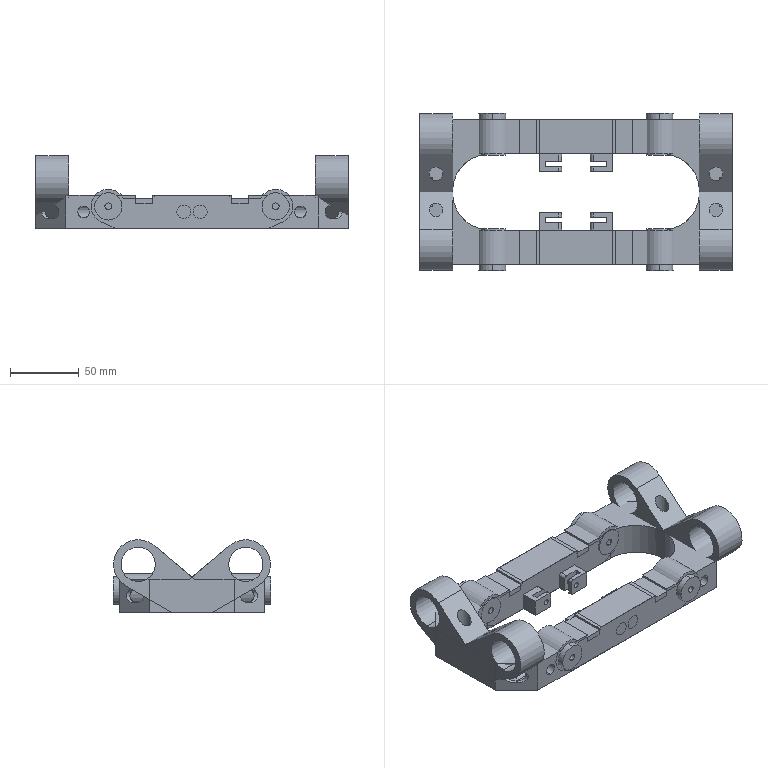NC program | Mastercam | posted with a generic post | part box 228 x 114.503 x 53 mm
Lines 3036 to 3656 of 11407:
(6 CHM |TOOL - 7|DIA. OFF. - 7|LEN. - 7|TOOL DIA. - 6.)
N6154 T7 M6
N6156 G0 G54 G90 X129.548 Y-5.75 C0. B0. S6000 M3
N6158 G43 H7 Z62.5
N6160 G81 G98 Z36.8 R39.5 F300.
N6162 G80
N6164 M5
N6166 G0 G28 G91 Z0.
N6168 G28
N6170 M01
N6172 G0 G17 G40 G80 G90 G94 G98
N6174 G0 G28 G91 Z0.
(12 FEM |TOOL - 12|DIA. OFF. - 12|LEN. - 12|TOOL DIA. - 12.)
N6176 T12 M6
N6178 G0 G54 G90 X164.238 Y26.324 C0. B0. S6000 M3
N6180 G43 H12 Z76.
N6182 Z31.
N6184 G1 Z25.5 F600.
N6186 X165.204 Y23.483 F6000.
N6188 G3 X168.044 Y21.449 I2.84 J.966
N6190 X169.01 Y21.609 J3.
N6192 G2 X175. Y22.6 I5.99 J-17.609
N6194 X193.6 Y4. J-18.6
N6196 X182.692 Y-12.935 I-18.6
N6198 G1 X172.523 Y-17.554
N6200 G3 X170.764 Y-20.285 I1.24 J-2.731
N6202 X171.032 Y-21.526 I2.999
N6204 G1 X172.272 Y-24.257
N6206 Z25. F600.
N6208 X171.032 Y-21.526 F6000.
N6210 G2 X170.763 Y-20.285 I2.731 J1.241
N6212 X172.523 Y-17.554 I3.
N6214 G1 X182.692 Y-12.935
N6216 G3 X193.6 Y4. I-7.692 J16.935
N6218 X175. Y22.6 I-18.6
N6220 X169.01 Y21.609 J-18.6
N6222 G2 X168.044 Y21.449 I-.966 J2.84
N6224 X165.204 Y23.483 J3.
N6226 G1 X164.238 Y26.324
N6228 Z24.5 F600.
N6230 X165.204 Y23.483 F6000.
N6232 G3 X168.044 Y21.449 I2.84 J.966
N6234 X169.01 Y21.609 J3.
N6236 G2 X175. Y22.6 I5.99 J-17.609
N6238 X193.6 Y4. J-18.6
N6240 X182.692 Y-12.935 I-18.6
N6242 G1 X172.523 Y-17.554
N6244 G3 X170.764 Y-20.285 I1.24 J-2.731
N6246 X171.032 Y-21.526 I2.999
N6248 G1 X172.272 Y-24.257
N6250 Z24. F600.
N6252 X171.032 Y-21.526 F6000.
N6254 G2 X170.763 Y-20.285 I2.731 J1.241
N6256 X172.523 Y-17.554 I3.
N6258 G1 X182.692 Y-12.935
N6260 G3 X193.6 Y4. I-7.692 J16.935
N6262 X175. Y22.6 I-18.6
N6264 X169.01 Y21.609 J-18.6
N6266 G2 X168.044 Y21.449 I-.966 J2.84
N6268 X165.204 Y23.483 J3.
N6270 G1 X164.238 Y26.324
N6272 Z23.5 F600.
N6274 X165.204 Y23.483 F6000.
N6276 G3 X168.044 Y21.449 I2.84 J.966
N6278 X169.01 Y21.609 J3.
N6280 G2 X175. Y22.6 I5.99 J-17.609
N6282 X193.6 Y4. J-18.6
N6284 X182.692 Y-12.935 I-18.6
N6286 G1 X172.523 Y-17.554
N6288 G3 X170.764 Y-20.285 I1.24 J-2.731
N6290 X171.032 Y-21.526 I2.999
N6292 G1 X172.272 Y-24.257
N6294 Z23. F600.
N6296 X171.032 Y-21.526 F6000.
N6298 G2 X170.763 Y-20.285 I2.731 J1.241
N6300 X172.523 Y-17.554 I3.
N6302 G1 X182.692 Y-12.935
N6304 G3 X193.6 Y4. I-7.692 J16.935
N6306 X175. Y22.6 I-18.6
N6308 X169.01 Y21.609 J-18.6
N6310 G2 X168.044 Y21.449 I-.966 J2.84
N6312 X165.204 Y23.483 J3.
N6314 G1 X164.238 Y26.324
N6316 Z22.5 F600.
N6318 X165.204 Y23.483 F6000.
N6320 G3 X168.044 Y21.449 I2.84 J.966
N6322 X169.01 Y21.609 J3.
N6324 G2 X175. Y22.6 I5.99 J-17.609
N6326 X193.6 Y4. J-18.6
N6328 X182.692 Y-12.935 I-18.6
N6330 G1 X172.523 Y-17.554
N6332 G3 X170.764 Y-20.285 I1.24 J-2.731
N6334 X171.032 Y-21.526 I2.999
N6336 G1 X172.272 Y-24.257
N6338 Z22. F600.
N6340 X171.032 Y-21.526 F6000.
N6342 G2 X170.763 Y-20.285 I2.731 J1.241
N6344 X172.523 Y-17.554 I3.
N6346 G1 X182.692 Y-12.935
N6348 G3 X193.6 Y4. I-7.692 J16.935
N6350 X175. Y22.6 I-18.6
N6352 X169.01 Y21.609 J-18.6
N6354 G2 X168.044 Y21.449 I-.966 J2.84
N6356 X165.204 Y23.483 J3.
N6358 G1 X164.238 Y26.324
N6360 Z21.5 F600.
N6362 X165.204 Y23.483 F6000.
N6364 G3 X168.044 Y21.449 I2.84 J.966
N6366 X169.01 Y21.609 J3.
N6368 G2 X175. Y22.6 I5.99 J-17.609
N6370 X193.6 Y4. J-18.6
N6372 X182.692 Y-12.935 I-18.6
N6374 G1 X172.523 Y-17.554
N6376 G3 X170.764 Y-20.285 I1.24 J-2.731
N6378 X171.032 Y-21.526 I2.999
N6380 G1 X172.272 Y-24.257
N6382 Z21. F600.
N6384 X171.032 Y-21.526 F6000.
N6386 G2 X170.763 Y-20.285 I2.731 J1.241
N6388 X172.523 Y-17.554 I3.
N6390 G1 X182.692 Y-12.935
N6392 G3 X193.6 Y4. I-7.692 J16.935
N6394 X175. Y22.6 I-18.6
N6396 X169.01 Y21.609 J-18.6
N6398 G2 X168.044 Y21.449 I-.966 J2.84
N6400 X165.204 Y23.483 J3.
N6402 G1 X164.238 Y26.324
N6404 Z20.5 F600.
N6406 X165.204 Y23.483 F6000.
N6408 G3 X168.044 Y21.449 I2.84 J.966
N6410 X169.01 Y21.609 J3.
N6412 G2 X175. Y22.6 I5.99 J-17.609
N6414 X193.6 Y4. J-18.6
N6416 X182.692 Y-12.935 I-18.6
N6418 G1 X172.523 Y-17.554
N6420 G3 X170.764 Y-20.285 I1.24 J-2.731
N6422 X171.032 Y-21.526 I2.999
N6424 G1 X172.272 Y-24.257
N6426 Z20. F600.
N6428 X171.032 Y-21.526 F6000.
N6430 G2 X170.763 Y-20.285 I2.731 J1.241
N6432 X172.523 Y-17.554 I3.
N6434 G1 X182.692 Y-12.935
N6436 G3 X193.6 Y4. I-7.692 J16.935
N6438 X175. Y22.6 I-18.6
N6440 X169.01 Y21.609 J-18.6
N6442 G2 X168.044 Y21.449 I-.966 J2.84
N6444 X165.204 Y23.483 J3.
N6446 G1 X164.238 Y26.324
N6448 Z19.5 F600.
N6450 X165.204 Y23.483 F6000.
N6452 G3 X168.044 Y21.449 I2.84 J.966
N6454 X169.01 Y21.609 J3.
N6456 G2 X175. Y22.6 I5.99 J-17.609
N6458 X193.6 Y4. J-18.6
N6460 X182.692 Y-12.935 I-18.6
N6462 G1 X172.523 Y-17.554
N6464 G3 X170.764 Y-20.285 I1.24 J-2.731
N6466 X171.032 Y-21.526 I2.999
N6468 G1 X172.272 Y-24.257
N6470 Z19. F600.
N6472 X171.032 Y-21.526 F6000.
N6474 G2 X170.763 Y-20.285 I2.731 J1.241
N6476 X172.523 Y-17.554 I3.
N6478 G1 X182.692 Y-12.935
N6480 G3 X193.6 Y4. I-7.692 J16.935
N6482 X175. Y22.6 I-18.6
N6484 X169.01 Y21.609 J-18.6
N6486 G2 X168.044 Y21.449 I-.966 J2.84
N6488 X165.204 Y23.483 J3.
N6490 G1 X164.238 Y26.324
N6492 Z18.5 F600.
N6494 X165.204 Y23.483 F6000.
N6496 G3 X168.044 Y21.449 I2.84 J.966
N6498 X169.01 Y21.609 J3.
N6500 G2 X175. Y22.6 I5.99 J-17.609
N6502 X193.6 Y4. J-18.6
N6504 X182.692 Y-12.935 I-18.6
N6506 G1 X172.523 Y-17.554
N6508 G3 X170.764 Y-20.285 I1.24 J-2.731
N6510 X171.032 Y-21.526 I2.999
N6512 G1 X172.272 Y-24.257
N6514 Z18. F600.
N6516 X171.032 Y-21.526 F6000.
N6518 G2 X170.763 Y-20.285 I2.731 J1.241
N6520 X172.523 Y-17.554 I3.
N6522 G1 X182.692 Y-12.935
N6524 G3 X193.6 Y4. I-7.692 J16.935
N6526 X175. Y22.6 I-18.6
N6528 X169.01 Y21.609 J-18.6
N6530 G2 X168.044 Y21.449 I-.966 J2.84
N6532 X165.204 Y23.483 J3.
N6534 G1 X164.238 Y26.324
N6536 Z17.5 F600.
N6538 X165.204 Y23.483 F6000.
N6540 G3 X168.044 Y21.449 I2.84 J.966
N6542 X169.01 Y21.609 J3.
N6544 G2 X175. Y22.6 I5.99 J-17.609
N6546 X193.6 Y4. J-18.6
N6548 X182.692 Y-12.935 I-18.6
N6550 G1 X172.523 Y-17.554
N6552 G3 X170.764 Y-20.285 I1.24 J-2.731
N6554 X171.032 Y-21.526 I2.999
N6556 G1 X172.272 Y-24.257
N6558 Z17. F600.
N6560 X171.032 Y-21.526 F6000.
N6562 G2 X170.763 Y-20.285 I2.731 J1.241
N6564 X172.523 Y-17.554 I3.
N6566 G1 X182.692 Y-12.935
N6568 G3 X193.6 Y4. I-7.692 J16.935
N6570 X175. Y22.6 I-18.6
N6572 X169.01 Y21.609 J-18.6
N6574 G2 X168.044 Y21.449 I-.966 J2.84
N6576 X165.204 Y23.483 J3.
N6578 G1 X164.238 Y26.324
N6580 Z16.5 F600.
N6582 X165.204 Y23.483 F6000.
N6584 G3 X168.044 Y21.449 I2.84 J.966
N6586 X169.01 Y21.609 J3.
N6588 G2 X175. Y22.6 I5.99 J-17.609
N6590 X193.6 Y4. J-18.6
N6592 X182.692 Y-12.935 I-18.6
N6594 G1 X172.523 Y-17.554
N6596 G3 X170.764 Y-20.285 I1.24 J-2.731
N6598 X171.032 Y-21.526 I2.999
N6600 G1 X172.272 Y-24.257
N6602 Z16. F600.
N6604 X171.032 Y-21.526 F6000.
N6606 G2 X170.763 Y-20.285 I2.731 J1.241
N6608 X172.523 Y-17.554 I3.
N6610 G1 X182.692 Y-12.935
N6612 G3 X193.6 Y4. I-7.692 J16.935
N6614 X175. Y22.6 I-18.6
N6616 X169.01 Y21.609 J-18.6
N6618 G2 X168.044 Y21.449 I-.966 J2.84
N6620 X165.204 Y23.483 J3.
N6622 G1 X164.238 Y26.324
N6624 Z15.5 F600.
N6626 X165.204 Y23.483 F6000.
N6628 G3 X168.044 Y21.449 I2.84 J.966
N6630 X169.01 Y21.609 J3.
N6632 G2 X175. Y22.6 I5.99 J-17.609
N6634 X193.6 Y4. J-18.6
N6636 X182.692 Y-12.935 I-18.6
N6638 G1 X172.523 Y-17.554
N6640 G3 X170.764 Y-20.285 I1.24 J-2.731
N6642 X171.032 Y-21.526 I2.999
N6644 G1 X172.272 Y-24.257
N6646 Z15. F600.
N6648 X171.032 Y-21.526 F6000.
N6650 G2 X170.763 Y-20.285 I2.731 J1.241
N6652 X172.523 Y-17.554 I3.
N6654 G1 X182.692 Y-12.935
N6656 G3 X193.6 Y4. I-7.692 J16.935
N6658 X175. Y22.6 I-18.6
N6660 X169.01 Y21.609 J-18.6
N6662 G2 X168.044 Y21.449 I-.966 J2.84
N6664 X165.204 Y23.483 J3.
N6666 G1 X164.238 Y26.324
N6668 Z14.5 F600.
N6670 X165.204 Y23.483 F6000.
N6672 G3 X168.044 Y21.449 I2.84 J.966
N6674 X169.01 Y21.609 J3.
N6676 G2 X175. Y22.6 I5.99 J-17.609
N6678 X193.6 Y4. J-18.6
N6680 X182.692 Y-12.935 I-18.6
N6682 G1 X172.523 Y-17.554
N6684 G3 X170.764 Y-20.285 I1.24 J-2.731
N6686 X171.032 Y-21.526 I2.999
N6688 G1 X172.272 Y-24.257
N6690 Z14. F600.
N6692 X171.032 Y-21.526 F6000.
N6694 G2 X170.763 Y-20.285 I2.731 J1.241
N6696 X172.523 Y-17.554 I3.
N6698 G1 X182.692 Y-12.935
N6700 G3 X193.6 Y4. I-7.692 J16.935
N6702 X175. Y22.6 I-18.6
N6704 X169.01 Y21.609 J-18.6
N6706 G2 X168.044 Y21.449 I-.966 J2.84
N6708 X165.204 Y23.483 J3.
N6710 G1 X164.238 Y26.324
N6712 Z13.5 F600.
N6714 X165.204 Y23.483 F6000.
N6716 G3 X168.044 Y21.449 I2.84 J.966
N6718 X169.01 Y21.609 J3.
N6720 G2 X175. Y22.6 I5.99 J-17.609
N6722 X193.6 Y4. J-18.6
N6724 X182.692 Y-12.935 I-18.6
N6726 G1 X172.523 Y-17.554
N6728 G3 X170.764 Y-20.285 I1.24 J-2.731
N6730 X171.032 Y-21.526 I2.999
N6732 G1 X172.272 Y-24.257
N6734 Z13. F600.
N6736 X171.032 Y-21.526 F6000.
N6738 G2 X170.763 Y-20.285 I2.731 J1.241
N6740 X172.523 Y-17.554 I3.
N6742 G1 X182.692 Y-12.935
N6744 G3 X193.6 Y4. I-7.692 J16.935
N6746 X175. Y22.6 I-18.6
N6748 X169.01 Y21.609 J-18.6
N6750 G2 X168.044 Y21.449 I-.966 J2.84
N6752 X165.204 Y23.483 J3.
N6754 G1 X164.238 Y26.324
N6756 Z12.5 F600.
N6758 X165.204 Y23.483 F6000.
N6760 G3 X168.044 Y21.449 I2.84 J.966
N6762 X169.01 Y21.609 J3.
N6764 G2 X175. Y22.6 I5.99 J-17.609
N6766 X193.6 Y4. J-18.6
N6768 X182.692 Y-12.935 I-18.6
N6770 G1 X172.523 Y-17.554
N6772 G3 X170.764 Y-20.285 I1.24 J-2.731
N6774 X171.032 Y-21.526 I2.999
N6776 G1 X172.272 Y-24.257
N6778 Z12. F600.
N6780 X171.032 Y-21.526 F6000.
N6782 G2 X170.763 Y-20.285 I2.731 J1.241
N6784 X172.523 Y-17.554 I3.
N6786 G1 X182.692 Y-12.935
N6788 G3 X193.6 Y4. I-7.692 J16.935
N6790 X175. Y22.6 I-18.6
N6792 X169.01 Y21.609 J-18.6
N6794 G2 X168.044 Y21.449 I-.966 J2.84
N6796 X165.204 Y23.483 J3.
N6798 G1 X164.238 Y26.324
N6800 Z11.5 F600.
N6802 X165.204 Y23.483 F6000.
N6804 G3 X168.044 Y21.449 I2.84 J.966
N6806 X169.01 Y21.609 J3.
N6808 G2 X175. Y22.6 I5.99 J-17.609
N6810 X193.6 Y4. J-18.6
N6812 X182.692 Y-12.935 I-18.6
N6814 G1 X172.523 Y-17.554
N6816 G3 X170.764 Y-20.285 I1.24 J-2.731
N6818 X171.032 Y-21.526 I2.999
N6820 G1 X172.272 Y-24.257
N6822 Z11. F600.
N6824 X171.032 Y-21.526 F6000.
N6826 G2 X170.763 Y-20.285 I2.731 J1.241
N6828 X172.523 Y-17.554 I3.
N6830 G1 X182.692 Y-12.935
N6832 G3 X193.6 Y4. I-7.692 J16.935
N6834 X175. Y22.6 I-18.6
N6836 X169.01 Y21.609 J-18.6
N6838 G2 X168.044 Y21.449 I-.966 J2.84
N6840 X165.204 Y23.483 J3.
N6842 G1 X164.238 Y26.324
N6844 Z10.5 F600.
N6846 X165.204 Y23.483 F6000.
N6848 G3 X168.044 Y21.449 I2.84 J.966
N6850 X169.01 Y21.609 J3.
N6852 G2 X175. Y22.6 I5.99 J-17.609
N6854 X193.6 Y4. J-18.6
N6856 X182.692 Y-12.935 I-18.6
N6858 G1 X172.523 Y-17.554
N6860 G3 X170.764 Y-20.285 I1.24 J-2.731
N6862 X171.032 Y-21.526 I2.999
N6864 G1 X172.272 Y-24.257
N6866 Z10. F600.
N6868 X171.032 Y-21.526 F6000.
N6870 G2 X170.763 Y-20.285 I2.731 J1.241
N6872 X172.523 Y-17.554 I3.
N6874 G1 X182.692 Y-12.935
N6876 G3 X193.6 Y4. I-7.692 J16.935
N6878 X175. Y22.6 I-18.6
N6880 X169.01 Y21.609 J-18.6
N6882 G2 X168.044 Y21.449 I-.966 J2.84
N6884 X165.204 Y23.483 J3.
N6886 G1 X164.238 Y26.324
N6888 Z9.5 F600.
N6890 X165.204 Y23.483 F6000.
N6892 G3 X168.044 Y21.449 I2.84 J.966
N6894 X169.01 Y21.609 J3.
N6896 G2 X175. Y22.6 I5.99 J-17.609
N6898 X193.6 Y4. J-18.6
N6900 X182.692 Y-12.935 I-18.6
N6902 G1 X172.523 Y-17.554
N6904 G3 X170.764 Y-20.285 I1.24 J-2.731
N6906 X171.032 Y-21.526 I2.999
N6908 G1 X172.272 Y-24.257
N6910 Z9. F600.
N6912 X171.032 Y-21.526 F6000.
N6914 G2 X170.763 Y-20.285 I2.731 J1.241
N6916 X172.523 Y-17.554 I3.
N6918 G1 X182.692 Y-12.935
N6920 G3 X193.6 Y4. I-7.692 J16.935
N6922 X175. Y22.6 I-18.6
N6924 X169.01 Y21.609 J-18.6
N6926 G2 X168.044 Y21.449 I-.966 J2.84
N6928 X165.204 Y23.483 J3.
N6930 G1 X164.238 Y26.324
N6932 Z8.5 F600.
N6934 X165.204 Y23.483 F6000.
N6936 G3 X168.044 Y21.449 I2.84 J.966
N6938 X169.01 Y21.609 J3.
N6940 G2 X175. Y22.6 I5.99 J-17.609
N6942 X193.6 Y4. J-18.6
N6944 X182.692 Y-12.935 I-18.6
N6946 G1 X172.523 Y-17.554
N6948 G3 X170.764 Y-20.285 I1.24 J-2.731
N6950 X171.032 Y-21.526 I2.999
N6952 G1 X172.272 Y-24.257
N6954 Z8. F600.
N6956 X171.032 Y-21.526 F6000.
N6958 G2 X170.763 Y-20.285 I2.731 J1.241
N6960 X172.523 Y-17.554 I3.
N6962 G1 X182.692 Y-12.935
N6964 G3 X193.6 Y4. I-7.692 J16.935
N6966 X175. Y22.6 I-18.6
N6968 X169.01 Y21.609 J-18.6
N6970 G2 X168.044 Y21.449 I-.966 J2.84
N6972 X165.204 Y23.483 J3.
N6974 G1 X164.238 Y26.324
N6976 Z7.5 F600.
N6978 X165.204 Y23.483 F6000.
N6980 G3 X168.044 Y21.449 I2.84 J.966
N6982 X169.01 Y21.609 J3.
N6984 G2 X175. Y22.6 I5.99 J-17.609
N6986 X193.6 Y4. J-18.6
N6988 X182.692 Y-12.935 I-18.6
N6990 G1 X172.523 Y-17.554
N6992 G3 X170.764 Y-20.285 I1.24 J-2.731
N6994 X171.032 Y-21.526 I2.999
N6996 G1 X172.272 Y-24.257
N6998 Z7. F600.
N7000 X171.032 Y-21.526 F6000.
N7002 G2 X170.763 Y-20.285 I2.731 J1.241
N7004 X172.523 Y-17.554 I3.
N7006 G1 X182.692 Y-12.935
N7008 G3 X193.6 Y4. I-7.692 J16.935
N7010 X175. Y22.6 I-18.6
N7012 X169.01 Y21.609 J-18.6
N7014 G2 X168.044 Y21.449 I-.966 J2.84
N7016 X165.204 Y23.483 J3.
N7018 G1 X164.238 Y26.324
N7020 Z6.5 F600.
N7022 X165.204 Y23.483 F6000.
N7024 G3 X168.044 Y21.449 I2.84 J.966
N7026 X169.01 Y21.609 J3.
N7028 G2 X175. Y22.6 I5.99 J-17.609
N7030 X193.6 Y4. J-18.6
N7032 X182.692 Y-12.935 I-18.6
N7034 G1 X172.523 Y-17.554
N7036 G3 X170.764 Y-20.285 I1.24 J-2.731
N7038 X171.032 Y-21.526 I2.999
N7040 G1 X172.272 Y-24.257
N7042 Z6. F600.
N7044 X171.032 Y-21.526 F6000.
N7046 G2 X170.763 Y-20.285 I2.731 J1.241
N7048 X172.523 Y-17.554 I3.
N7050 G1 X182.692 Y-12.935
N7052 G3 X193.6 Y4. I-7.692 J16.935
N7054 X175. Y22.6 I-18.6
N7056 X169.01 Y21.609 J-18.6
N7058 G2 X168.044 Y21.449 I-.966 J2.84
N7060 X165.204 Y23.483 J3.
N7062 G1 X164.238 Y26.324
N7064 Z5.5 F600.
N7066 X165.204 Y23.483 F6000.
N7068 G3 X168.044 Y21.449 I2.84 J.966
N7070 X169.01 Y21.609 J3.
N7072 G2 X175. Y22.6 I5.99 J-17.609
N7074 X193.6 Y4. J-18.6
N7076 X182.692 Y-12.935 I-18.6
N7078 G1 X172.523 Y-17.554
N7080 G3 X170.764 Y-20.285 I1.24 J-2.731
N7082 X171.032 Y-21.526 I2.999
N7084 G1 X172.272 Y-24.257
N7086 Z5. F600.
N7088 X171.032 Y-21.526 F6000.
N7090 G2 X170.763 Y-20.285 I2.731 J1.241
N7092 X172.523 Y-17.554 I3.
N7094 G1 X182.692 Y-12.935
N7096 G3 X193.6 Y4. I-7.692 J16.935
N7098 X175. Y22.6 I-18.6
N7100 X169.01 Y21.609 J-18.6
N7102 G2 X168.044 Y21.449 I-.966 J2.84
N7104 X165.204 Y23.483 J3.
N7106 G1 X164.238 Y26.324
N7108 Z4.5 F600.
N7110 X165.204 Y23.483 F6000.
N7112 G3 X168.044 Y21.449 I2.84 J.966
N7114 X169.01 Y21.609 J3.
N7116 G2 X175. Y22.6 I5.99 J-17.609
N7118 X193.6 Y4. J-18.6
N7120 X182.692 Y-12.935 I-18.6
N7122 G1 X172.523 Y-17.554
N7124 G3 X170.764 Y-20.285 I1.24 J-2.731
N7126 X171.032 Y-21.526 I2.999
N7128 G1 X172.272 Y-24.257
N7130 Z4. F600.
N7132 X171.032 Y-21.526 F6000.
N7134 G2 X170.763 Y-20.285 I2.731 J1.241
N7136 X172.523 Y-17.554 I3.
N7138 G1 X182.692 Y-12.935
N7140 G3 X193.6 Y4. I-7.692 J16.935
N7142 X175. Y22.6 I-18.6
N7144 X169.01 Y21.609 J-18.6
N7146 G2 X168.044 Y21.449 I-.966 J2.84
N7148 X165.204 Y23.483 J3.
N7150 G1 X164.238 Y26.324
N7152 Z3.5 F600.
N7154 X165.204 Y23.483 F6000.
N7156 G3 X168.044 Y21.449 I2.84 J.966
N7158 X169.01 Y21.609 J3.
N7160 G2 X175. Y22.6 I5.99 J-17.609
N7162 X193.6 Y4. J-18.6
N7164 X182.692 Y-12.935 I-18.6
N7166 G1 X172.523 Y-17.554
N7168 G3 X170.764 Y-20.285 I1.24 J-2.731
N7170 X171.032 Y-21.526 I2.999
N7172 G1 X172.272 Y-24.257
N7174 Z3. F600.
N7176 X171.032 Y-21.526 F6000.
N7178 G2 X170.763 Y-20.285 I2.731 J1.241
N7180 X172.523 Y-17.554 I3.
N7182 G1 X182.692 Y-12.935
N7184 G3 X193.6 Y4. I-7.692 J16.935
N7186 X175. Y22.6 I-18.6
N7188 X169.01 Y21.609 J-18.6
N7190 G2 X168.044 Y21.449 I-.966 J2.84
N7192 X165.204 Y23.483 J3.
N7194 G1 X164.238 Y26.324
N7196 Z2.5 F600.
N7198 X165.204 Y23.483 F6000.
N7200 G3 X168.044 Y21.449 I2.84 J.966
N7202 X169.01 Y21.609 J3.
N7204 G2 X175. Y22.6 I5.99 J-17.609
N7206 X193.6 Y4. J-18.6
N7208 X182.692 Y-12.935 I-18.6
N7210 G1 X172.523 Y-17.554
N7212 G3 X170.764 Y-20.285 I1.24 J-2.731
N7214 X171.032 Y-21.526 I2.999
N7216 G1 X172.272 Y-24.257
N7218 Z2. F600.
N7220 X171.032 Y-21.526 F6000.
N7222 G2 X170.763 Y-20.285 I2.731 J1.241
N7224 X172.523 Y-17.554 I3.
N7226 G1 X182.692 Y-12.935
N7228 G3 X193.6 Y4. I-7.692 J16.935
N7230 X175. Y22.6 I-18.6
N7232 X169.01 Y21.609 J-18.6
N7234 G2 X168.044 Y21.449 I-.966 J2.84
N7236 X165.204 Y23.483 J3.
N7238 G1 X164.238 Y26.324
N7240 Z1.5 F600.
N7242 X165.204 Y23.483 F6000.
N7244 G3 X168.044 Y21.449 I2.84 J.966
N7246 X169.01 Y21.609 J3.
N7248 G2 X175. Y22.6 I5.99 J-17.609
N7250 X193.6 Y4. J-18.6
N7252 X182.692 Y-12.935 I-18.6
N7254 G1 X172.523 Y-17.554
N7256 G3 X170.764 Y-20.285 I1.24 J-2.731
N7258 X171.032 Y-21.526 I2.999
N7260 G1 X172.272 Y-24.257
N7262 Z1. F600.
N7264 X171.032 Y-21.526 F6000.
N7266 G2 X170.763 Y-20.285 I2.731 J1.241
N7268 X172.523 Y-17.554 I3.
N7270 G1 X182.692 Y-12.935
N7272 G3 X193.6 Y4. I-7.692 J16.935
N7274 X175. Y22.6 I-18.6
N7276 X169.01 Y21.609 J-18.6
N7278 G2 X168.044 Y21.449 I-.966 J2.84
N7280 X165.204 Y23.483 J3.
N7282 G1 X164.238 Y26.324
N7284 Z.5 F600.
N7286 X165.204 Y23.483 F6000.
N7288 G3 X168.044 Y21.449 I2.84 J.966
N7290 X169.01 Y21.609 J3.
N7292 G2 X175. Y22.6 I5.99 J-17.609
N7294 X193.6 Y4. J-18.6
N7296 X182.692 Y-12.935 I-18.6
N7298 G1 X172.523 Y-17.554
N7300 G3 X170.764 Y-20.285 I1.24 J-2.731
N7302 X171.032 Y-21.526 I2.999
N7304 G1 X172.272 Y-24.257
N7306 Z0. F600.
N7308 X171.032 Y-21.526 F6000.
N7310 G2 X170.763 Y-20.285 I2.731 J1.241
N7312 X172.523 Y-17.554 I3.
N7314 G1 X182.692 Y-12.935
N7316 G3 X193.6 Y4. I-7.692 J16.935
N7318 X175. Y22.6 I-18.6
N7320 X169.01 Y21.609 J-18.6
N7322 G2 X168.044 Y21.449 I-.966 J2.84
N7324 X165.204 Y23.483 J3.
N7326 G1 X164.238 Y26.324
N7328 Z-.5 F600.
N7330 X165.204 Y23.483 F6000.
N7332 G3 X168.044 Y21.449 I2.84 J.966
N7334 X169.01 Y21.609 J3.
N7336 G2 X175. Y22.6 I5.99 J-17.609
N7338 X193.6 Y4. J-18.6
N7340 X182.692 Y-12.935 I-18.6
N7342 G1 X172.523 Y-17.554
N7344 G3 X170.764 Y-20.285 I1.24 J-2.731
N7346 X171.032 Y-21.526 I2.999
N7348 G1 X172.272 Y-24.257
N7350 G0 Z76.
N7352 X164.27 Y26.229
N7354 Z31.
N7356 G1 Z-.5 F600.
N7358 X165.236 Y23.389 F1000.
N7360 G3 X168.076 Y21.355 I2.84 J.966
N7362 X169.043 Y21.515 J3.
N7364 G2 X175. Y22.5 I5.957 J-17.515
N7366 X193.5 Y4. J-18.5
N7368 X182.651 Y-12.844 I-18.5
N7370 G1 X172.481 Y-17.463
N7372 G3 X170.722 Y-20.194 I1.241 J-2.731
N7374 X170.99 Y-21.435 I3.
N7376 G1 X172.231 Y-24.166
N7378 G0 Z76.
N7380 M5
N7382 G0 G28 G91 Z0.
N7384 G28
N7386 M01
N7388 G0 G17 G40 G80 G90 G94 G98
N7390 G0 G28 G91 Z0.